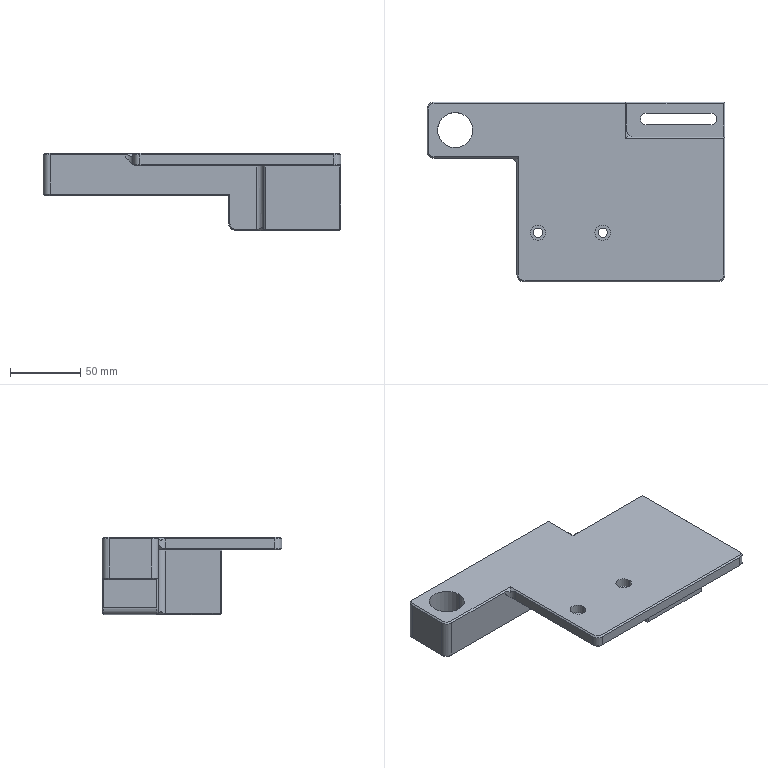Part | 1 solid | 89 faces | box 212 x 128 x 55 mm | volume 472806 mm3 | plane 51 | cylinder 26 | cone 12 | commonest cylinder face diameters 10 x8 6.6 x4 11 x4 8.2 x3 14 x3 6.8 x2